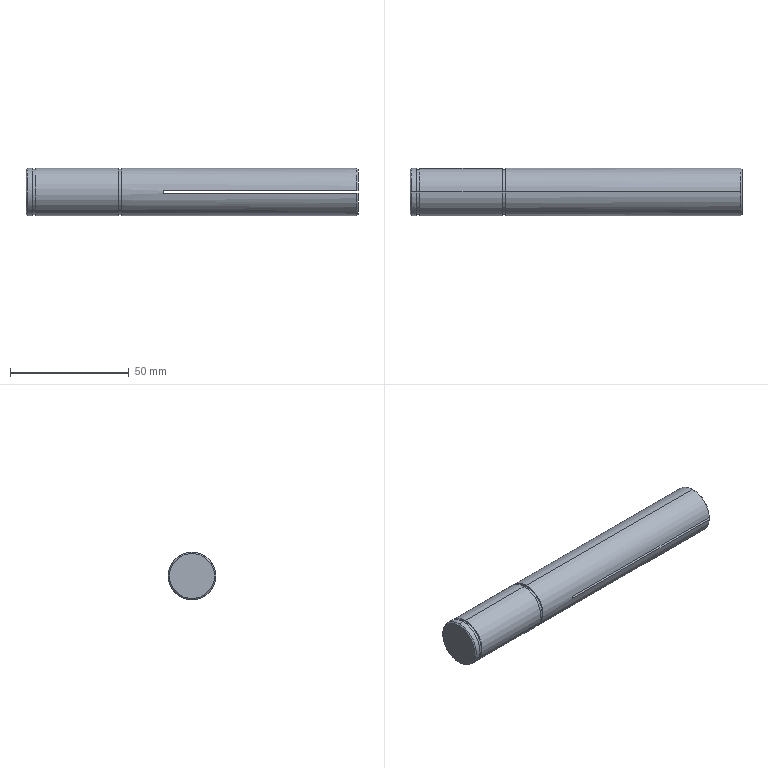Part | NX | 1 solid | 24 faces | box 140 x 20 x 20 mm | volume 42079 mm3 | plane 10 | cylinder 10 | cone 4 | commonest cylinder face diameters 20 x6 19 x4
STEP:
#1=CARTESIAN_POINT('',(0.,-9.5,0.));
#2=VERTEX_POINT('',#1);
#3=CARTESIAN_POINT('',(0.,9.5,0.));
#4=VERTEX_POINT('',#3);
#5=CARTESIAN_POINT('',(0.,0.,0.));
#6=DIRECTION('',(-1.,0.,0.));
#7=DIRECTION('',(0.,0.,-1.));
#8=AXIS2_PLACEMENT_3D('',#5,#6,#7);
#9=CIRCLE('',#8,9.5);
#10=EDGE_CURVE('',#2,#4,#9,.T.);
#11=ORIENTED_EDGE('',*,*,#10,.T.);
#12=CARTESIAN_POINT('',(0.,0.,0.));
#13=DIRECTION('',(-1.,0.,0.));
#14=DIRECTION('',(0.,0.,-1.));
#15=AXIS2_PLACEMENT_3D('',#12,#13,#14);
#16=CIRCLE('',#15,9.5);
#17=EDGE_CURVE('',#4,#2,#16,.T.);
#18=ORIENTED_EDGE('',*,*,#17,.T.);
#19=EDGE_LOOP('',(#11,#18));
#20=FACE_BOUND('',#19,.T.);
#21=CARTESIAN_POINT('',(0.,0.,0.));
#22=DIRECTION('',(1.,0.,0.));
#23=DIRECTION('',(0.,1.,0.));
#24=AXIS2_PLACEMENT_3D('',#21,#22,#23);
#25=PLANE('',#24);
#26=ADVANCED_FACE('',(#20),#25,.F.);
#27=ORIENTED_EDGE('',*,*,#10,.F.);
#28=CARTESIAN_POINT('',(0.5,-10.,0.));
#29=VERTEX_POINT('',#28);
#30=CARTESIAN_POINT('',(0.25,-9.75,0.));
#31=DIRECTION('',(0.7071,-0.7071,0.));
#32=VECTOR('',#31,1000.);
#33=LINE('',#30,#32);
#34=EDGE_CURVE('',#29,#2,#33,.F.);
#35=ORIENTED_EDGE('',*,*,#34,.F.);
#36=CARTESIAN_POINT('',(0.5,0.,10.));
#37=VERTEX_POINT('',#36);
#38=CARTESIAN_POINT('',(0.5,0.,0.));
#39=DIRECTION('',(-1.,0.,0.));
#40=DIRECTION('',(0.,0.,-1.));
#41=AXIS2_PLACEMENT_3D('',#38,#39,#40);
#42=CIRCLE('',#41,10.);
#43=EDGE_CURVE('',#29,#37,#42,.T.);
#44=ORIENTED_EDGE('',*,*,#43,.T.);
#45=CARTESIAN_POINT('',(0.5,10.,0.));
#46=VERTEX_POINT('',#45);
#47=CARTESIAN_POINT('',(0.5,0.,0.));
#48=DIRECTION('',(-1.,0.,0.));
#49=DIRECTION('',(0.,0.,-1.));
#50=AXIS2_PLACEMENT_3D('',#47,#48,#49);
#51=CIRCLE('',#50,10.);
#52=EDGE_CURVE('',#37,#46,#51,.T.);
#53=ORIENTED_EDGE('',*,*,#52,.T.);
#54=CARTESIAN_POINT('',(0.25,9.75,0.));
#55=DIRECTION('',(0.7071,0.7071,0.));
#56=VECTOR('',#55,1000.);
#57=LINE('',#54,#56);
#58=EDGE_CURVE('',#46,#4,#57,.F.);
#59=ORIENTED_EDGE('',*,*,#58,.T.);
#60=EDGE_LOOP('',(#27,#35,#44,#53,#59));
#61=FACE_BOUND('',#60,.T.);
#62=CARTESIAN_POINT('',(0.25,0.,0.));
#63=DIRECTION('',(1.,0.,0.));
#64=DIRECTION('',(0.,-1.,0.));
#65=AXIS2_PLACEMENT_3D('',#62,#63,#64);
#66=CONICAL_SURFACE('',#65,9.75,0.7854);
#67=ADVANCED_FACE('',(#61),#66,.T.);
#68=CARTESIAN_POINT('',(2.65,0.,-10.));
#69=VERTEX_POINT('',#68);
#70=CARTESIAN_POINT('',(2.65,0.,10.));
#71=VERTEX_POINT('',#70);
#72=CARTESIAN_POINT('',(2.65,0.,0.));
#73=DIRECTION('',(1.,0.,0.));
#74=DIRECTION('',(0.,0.,1.));
#75=AXIS2_PLACEMENT_3D('',#72,#73,#74);
#76=CIRCLE('',#75,10.);
#77=EDGE_CURVE('',#69,#71,#76,.T.);
#78=ORIENTED_EDGE('',*,*,#77,.F.);
#79=CARTESIAN_POINT('',(0.5,0.,-10.));
#80=VERTEX_POINT('',#79);
#81=CARTESIAN_POINT('',(147.,0.,-10.));
#82=DIRECTION('',(-1.,0.,0.));
#83=VECTOR('',#82,1000.);
#84=LINE('',#81,#83);
#85=EDGE_CURVE('',#80,#69,#84,.F.);
#86=ORIENTED_EDGE('',*,*,#85,.F.);
#87=CARTESIAN_POINT('',(0.5,0.,0.));
#88=DIRECTION('',(-1.,0.,0.));
#89=DIRECTION('',(0.,0.,-1.));
#90=AXIS2_PLACEMENT_3D('',#87,#88,#89);
#91=CIRCLE('',#90,10.);
#92=EDGE_CURVE('',#46,#80,#91,.T.);
#93=ORIENTED_EDGE('',*,*,#92,.F.);
#94=ORIENTED_EDGE('',*,*,#52,.F.);
#95=CARTESIAN_POINT('',(147.,0.,10.));
#96=DIRECTION('',(-1.,0.,0.));
#97=VECTOR('',#96,1000.);
#98=LINE('',#95,#97);
#99=EDGE_CURVE('',#37,#71,#98,.F.);
#100=ORIENTED_EDGE('',*,*,#99,.T.);
#101=EDGE_LOOP('',(#78,#86,#93,#94,#100));
#102=FACE_BOUND('',#101,.T.);
#103=CARTESIAN_POINT('',(147.,0.,0.));
#104=DIRECTION('',(-1.,0.,0.));
#105=DIRECTION('',(0.,0.,-1.));
#106=AXIS2_PLACEMENT_3D('',#103,#104,#105);
#107=CYLINDRICAL_SURFACE('',#106,10.);
#108=ADVANCED_FACE('',(#102),#107,.T.);
#109=CARTESIAN_POINT('',(140.,-9.484,-0.55));
#110=VERTEX_POINT('',#109);
#111=CARTESIAN_POINT('',(140.,9.484,-0.55));
#112=VERTEX_POINT('',#111);
#113=CARTESIAN_POINT('',(140.,0.,-0.55));
#114=DIRECTION('',(0.,1.,0.));
#115=VECTOR('',#114,1000.);
#116=LINE('',#113,#115);
#117=EDGE_CURVE('',#110,#112,#116,.T.);
#118=ORIENTED_EDGE('',*,*,#117,.F.);
#119=CARTESIAN_POINT('',(140.,0.,0.));
#120=DIRECTION('',(1.,0.,0.));
#121=DIRECTION('',(0.,1.,0.));
#122=AXIS2_PLACEMENT_3D('',#119,#120,#121);
#123=CIRCLE('',#122,9.5);
#124=EDGE_CURVE('',#110,#112,#123,.T.);
#125=ORIENTED_EDGE('',*,*,#124,.T.);
#126=EDGE_LOOP('',(#118,#125));
#127=FACE_BOUND('',#126,.T.);
#128=CARTESIAN_POINT('',(140.,0.,0.));
#129=DIRECTION('',(1.,0.,0.));
#130=DIRECTION('',(0.,1.,0.));
#131=AXIS2_PLACEMENT_3D('',#128,#129,#130);
#132=PLANE('',#131);
#133=ADVANCED_FACE('',(#127),#132,.T.);
#134=CARTESIAN_POINT('',(140.,9.484,0.55));
#135=VERTEX_POINT('',#134);
#136=CARTESIAN_POINT('',(140.,-9.484,0.55));
#137=VERTEX_POINT('',#136);
#138=CARTESIAN_POINT('',(140.,0.,0.55));
#139=DIRECTION('',(0.,-1.,0.));
#140=VECTOR('',#139,1000.);
#141=LINE('',#138,#140);
#142=EDGE_CURVE('',#135,#137,#141,.T.);
#143=ORIENTED_EDGE('',*,*,#142,.F.);
#144=CARTESIAN_POINT('',(140.,0.,0.));
#145=DIRECTION('',(1.,0.,0.));
#146=DIRECTION('',(0.,1.,0.));
#147=AXIS2_PLACEMENT_3D('',#144,#145,#146);
#148=CIRCLE('',#147,9.5);
#149=EDGE_CURVE('',#135,#137,#148,.T.);
#150=ORIENTED_EDGE('',*,*,#149,.T.);
#151=EDGE_LOOP('',(#143,#150));
#152=FACE_BOUND('',#151,.T.);
#153=CARTESIAN_POINT('',(140.,0.,0.));
#154=DIRECTION('',(1.,0.,0.));
#155=DIRECTION('',(0.,1.,0.));
#156=AXIS2_PLACEMENT_3D('',#153,#154,#155);
#157=PLANE('',#156);
#158=ADVANCED_FACE('',(#152),#157,.T.);
#159=ORIENTED_EDGE('',*,*,#77,.T.);
#160=CARTESIAN_POINT('',(2.65,0.,0.));
#161=DIRECTION('',(1.,0.,0.));
#162=DIRECTION('',(0.,0.,1.));
#163=AXIS2_PLACEMENT_3D('',#160,#161,#162);
#164=CIRCLE('',#163,10.);
#165=EDGE_CURVE('',#71,#69,#164,.T.);
#166=ORIENTED_EDGE('',*,*,#165,.T.);
#167=EDGE_LOOP('',(#159,#166));
#168=FACE_BOUND('',#167,.T.);
#169=CARTESIAN_POINT('',(2.65,0.,-9.5));
#170=VERTEX_POINT('',#169);
#171=CARTESIAN_POINT('',(2.65,0.,9.5));
#172=VERTEX_POINT('',#171);
#173=CARTESIAN_POINT('',(2.65,0.,0.));
#174=DIRECTION('',(-1.,0.,0.));
#175=DIRECTION('',(0.,0.,-1.));
#176=AXIS2_PLACEMENT_3D('',#173,#174,#175);
#177=CIRCLE('',#176,9.5);
#178=EDGE_CURVE('',#170,#172,#177,.T.);
#179=ORIENTED_EDGE('',*,*,#178,.T.);
#180=CARTESIAN_POINT('',(2.65,0.,0.));
#181=DIRECTION('',(-1.,0.,0.));
#182=DIRECTION('',(0.,0.,-1.));
#183=AXIS2_PLACEMENT_3D('',#180,#181,#182);
#184=CIRCLE('',#183,9.5);
#185=EDGE_CURVE('',#172,#170,#184,.T.);
#186=ORIENTED_EDGE('',*,*,#185,.T.);
#187=EDGE_LOOP('',(#179,#186));
#188=FACE_BOUND('',#187,.T.);
#189=CARTESIAN_POINT('',(2.65,0.,0.));
#190=DIRECTION('',(1.,0.,0.));
#191=DIRECTION('',(0.,1.,0.));
#192=AXIS2_PLACEMENT_3D('',#189,#190,#191);
#193=PLANE('',#192);
#194=ADVANCED_FACE('',(#168,#188),#193,.T.);
#195=ORIENTED_EDGE('',*,*,#178,.F.);
#196=CARTESIAN_POINT('',(4.,0.,-9.5));
#197=VERTEX_POINT('',#196);
#198=CARTESIAN_POINT('',(147.,0.,-9.5));
#199=DIRECTION('',(-1.,0.,0.));
#200=VECTOR('',#199,1000.);
#201=LINE('',#198,#200);
#202=EDGE_CURVE('',#170,#197,#201,.F.);
#203=ORIENTED_EDGE('',*,*,#202,.T.);
#204=CARTESIAN_POINT('',(4.,0.,9.5));
#205=VERTEX_POINT('',#204);
#206=CARTESIAN_POINT('',(4.,0.,0.));
#207=DIRECTION('',(1.,0.,0.));
#208=DIRECTION('',(0.,0.,1.));
#209=AXIS2_PLACEMENT_3D('',#206,#207,#208);
#210=CIRCLE('',#209,9.5);
#211=EDGE_CURVE('',#205,#197,#210,.T.);
#212=ORIENTED_EDGE('',*,*,#211,.F.);
#213=CARTESIAN_POINT('',(147.,0.,9.5));
#214=DIRECTION('',(-1.,0.,0.));
#215=VECTOR('',#214,1000.);
#216=LINE('',#213,#215);
#217=EDGE_CURVE('',#172,#205,#216,.F.);
#218=ORIENTED_EDGE('',*,*,#217,.F.);
#219=EDGE_LOOP('',(#195,#203,#212,#218));
#220=FACE_BOUND('',#219,.T.);
#221=CARTESIAN_POINT('',(147.,0.,0.));
#222=DIRECTION('',(-1.,0.,0.));
#223=DIRECTION('',(0.,0.,-1.));
#224=AXIS2_PLACEMENT_3D('',#221,#222,#223);
#225=CYLINDRICAL_SURFACE('',#224,9.5);
#226=ADVANCED_FACE('',(#220),#225,.T.);
#227=CARTESIAN_POINT('',(139.5,-9.985,0.55));
#228=VERTEX_POINT('',#227);
#229=CARTESIAN_POINT('',(139.5,-9.985,0.55));
#230=CARTESIAN_POINT('',(139.542,-9.943,0.55));
#231=CARTESIAN_POINT('',(139.583,-9.901,0.55));
#232=CARTESIAN_POINT('',(139.625,-9.86,0.55));
#233=CARTESIAN_POINT('',(139.667,-9.818,0.55));
#234=CARTESIAN_POINT('',(139.708,-9.776,0.55));
#235=CARTESIAN_POINT('',(139.75,-9.734,0.55));
#236=CARTESIAN_POINT('',(139.792,-9.693,0.55));
#237=CARTESIAN_POINT('',(139.833,-9.651,0.55));
#238=CARTESIAN_POINT('',(139.875,-9.609,0.55));
#239=CARTESIAN_POINT('',(139.917,-9.568,0.55));
#240=CARTESIAN_POINT('',(139.958,-9.526,0.55));
#241=CARTESIAN_POINT('',(140.,-9.484,0.55));
#242=B_SPLINE_CURVE_WITH_KNOTS('',3,(#229,#230,#231,#232,#233,#234,#235,#236,#237,#238,#239,#240,#241),.UNSPECIFIED.,.F.,.F.,(4,3,3,3,4),(0.,0.1769,0.3538,0.5308,0.7077),.UNSPECIFIED.);
#243=EDGE_CURVE('',#228,#137,#242,.T.);
#244=ORIENTED_EDGE('',*,*,#243,.F.);
#245=CARTESIAN_POINT('',(57.9,-9.985,0.55));
#246=VERTEX_POINT('',#245);
#247=CARTESIAN_POINT('',(147.,-9.985,0.55));
#248=DIRECTION('',(-1.,0.,0.));
#249=VECTOR('',#248,1000.);
#250=LINE('',#247,#249);
#251=EDGE_CURVE('',#228,#246,#250,.T.);
#252=ORIENTED_EDGE('',*,*,#251,.T.);
#253=CARTESIAN_POINT('',(57.9,9.985,0.55));
#254=VERTEX_POINT('',#253);
#255=CARTESIAN_POINT('',(57.9,0.,0.55));
#256=DIRECTION('',(0.,-1.,0.));
#257=VECTOR('',#256,1000.);
#258=LINE('',#255,#257);
#259=EDGE_CURVE('',#254,#246,#258,.T.);
#260=ORIENTED_EDGE('',*,*,#259,.F.);
#261=CARTESIAN_POINT('',(139.5,9.985,0.55));
#262=VERTEX_POINT('',#261);
#263=CARTESIAN_POINT('',(147.,9.985,0.55));
#264=DIRECTION('',(-1.,0.,0.));
#265=VECTOR('',#264,1000.);
#266=LINE('',#263,#265);
#267=EDGE_CURVE('',#262,#254,#266,.T.);
#268=ORIENTED_EDGE('',*,*,#267,.F.);
#269=CARTESIAN_POINT('',(140.,9.484,0.55));
#270=CARTESIAN_POINT('',(139.958,9.526,0.55));
#271=CARTESIAN_POINT('',(139.917,9.568,0.55));
#272=CARTESIAN_POINT('',(139.875,9.609,0.55));
#273=CARTESIAN_POINT('',(139.833,9.651,0.55));
#274=CARTESIAN_POINT('',(139.792,9.693,0.55));
#275=CARTESIAN_POINT('',(139.75,9.734,0.55));
#276=CARTESIAN_POINT('',(139.708,9.776,0.55));
#277=CARTESIAN_POINT('',(139.667,9.818,0.55));
#278=CARTESIAN_POINT('',(139.625,9.86,0.55));
#279=CARTESIAN_POINT('',(139.583,9.901,0.55));
#280=CARTESIAN_POINT('',(139.542,9.943,0.55));
#281=CARTESIAN_POINT('',(139.5,9.985,0.55));
#282=B_SPLINE_CURVE_WITH_KNOTS('',3,(#269,#270,#271,#272,#273,#274,#275,#276,#277,#278,#279,#280,#281),.UNSPECIFIED.,.F.,.F.,(4,3,3,3,4),(0.,0.1769,0.3538,0.5308,0.7077),.UNSPECIFIED.);
#283=EDGE_CURVE('',#135,#262,#282,.T.);
#284=ORIENTED_EDGE('',*,*,#283,.F.);
#285=ORIENTED_EDGE('',*,*,#142,.T.);
#286=EDGE_LOOP('',(#244,#252,#260,#268,#284,#285));
#287=FACE_BOUND('',#286,.T.);
#288=CARTESIAN_POINT('',(140.,-10.978,0.55));
#289=DIRECTION('',(0.,0.,-1.));
#290=DIRECTION('',(0.,-1.,0.));
#291=AXIS2_PLACEMENT_3D('',#288,#289,#290);
#292=PLANE('',#291);
#293=ADVANCED_FACE('',(#287),#292,.T.);
#294=CARTESIAN_POINT('',(4.,0.,10.));
#295=VERTEX_POINT('',#294);
#296=CARTESIAN_POINT('',(4.,0.,-10.));
#297=VERTEX_POINT('',#296);
#298=CARTESIAN_POINT('',(4.,0.,0.));
#299=DIRECTION('',(-1.,0.,0.));
#300=DIRECTION('',(0.,0.,-1.));
#301=AXIS2_PLACEMENT_3D('',#298,#299,#300);
#302=CIRCLE('',#301,10.);
#303=EDGE_CURVE('',#295,#297,#302,.T.);
#304=ORIENTED_EDGE('',*,*,#303,.T.);
#305=CARTESIAN_POINT('',(4.,0.,0.));
#306=DIRECTION('',(-1.,0.,0.));
#307=DIRECTION('',(0.,0.,-1.));
#308=AXIS2_PLACEMENT_3D('',#305,#306,#307);
#309=CIRCLE('',#308,10.);
#310=EDGE_CURVE('',#297,#295,#309,.T.);
#311=ORIENTED_EDGE('',*,*,#310,.T.);
#312=EDGE_LOOP('',(#304,#311));
#313=FACE_BOUND('',#312,.T.);
#314=CARTESIAN_POINT('',(4.,0.,0.));
#315=DIRECTION('',(1.,0.,0.));
#316=DIRECTION('',(0.,0.,1.));
#317=AXIS2_PLACEMENT_3D('',#314,#315,#316);
#318=CIRCLE('',#317,9.5);
#319=EDGE_CURVE('',#197,#205,#318,.T.);
#320=ORIENTED_EDGE('',*,*,#319,.T.);
#321=ORIENTED_EDGE('',*,*,#211,.T.);
#322=EDGE_LOOP('',(#320,#321));
#323=FACE_BOUND('',#322,.T.);
#324=CARTESIAN_POINT('',(4.,0.,0.));
#325=DIRECTION('',(1.,0.,0.));
#326=DIRECTION('',(0.,1.,0.));
#327=AXIS2_PLACEMENT_3D('',#324,#325,#326);
#328=PLANE('',#327);
#329=ADVANCED_FACE('',(#313,#323),#328,.F.);
#330=ORIENTED_EDGE('',*,*,#303,.F.);
#331=CARTESIAN_POINT('',(39.,0.,10.));
#332=VERTEX_POINT('',#331);
#333=CARTESIAN_POINT('',(147.,0.,10.));
#334=DIRECTION('',(-1.,0.,0.));
#335=VECTOR('',#334,1000.);
#336=LINE('',#333,#335);
#337=EDGE_CURVE('',#332,#295,#336,.T.);
#338=ORIENTED_EDGE('',*,*,#337,.F.);
#339=CARTESIAN_POINT('',(39.,0.,-10.));
#340=VERTEX_POINT('',#339);
#341=CARTESIAN_POINT('',(39.,0.,0.));
#342=DIRECTION('',(1.,0.,0.));
#343=DIRECTION('',(0.,0.,1.));
#344=AXIS2_PLACEMENT_3D('',#341,#342,#343);
#345=CIRCLE('',#344,10.);
#346=EDGE_CURVE('',#340,#332,#345,.T.);
#347=ORIENTED_EDGE('',*,*,#346,.F.);
#348=CARTESIAN_POINT('',(147.,0.,-10.));
#349=DIRECTION('',(-1.,0.,0.));
#350=VECTOR('',#349,1000.);
#351=LINE('',#348,#350);
#352=EDGE_CURVE('',#340,#297,#351,.T.);
#353=ORIENTED_EDGE('',*,*,#352,.T.);
#354=EDGE_LOOP('',(#330,#338,#347,#353));
#355=FACE_BOUND('',#354,.T.);
#356=CARTESIAN_POINT('',(147.,0.,0.));
#357=DIRECTION('',(-1.,0.,0.));
#358=DIRECTION('',(0.,0.,-1.));
#359=AXIS2_PLACEMENT_3D('',#356,#357,#358);
#360=CYLINDRICAL_SURFACE('',#359,10.);
#361=ADVANCED_FACE('',(#355),#360,.T.);
#362=CARTESIAN_POINT('',(139.5,9.985,-0.55));
#363=VERTEX_POINT('',#362);
#364=CARTESIAN_POINT('',(139.5,9.985,-0.55));
#365=CARTESIAN_POINT('',(139.542,9.943,-0.55));
#366=CARTESIAN_POINT('',(139.583,9.901,-0.55));
#367=CARTESIAN_POINT('',(139.625,9.86,-0.55));
#368=CARTESIAN_POINT('',(139.667,9.818,-0.55));
#369=CARTESIAN_POINT('',(139.708,9.776,-0.55));
#370=CARTESIAN_POINT('',(139.75,9.734,-0.55));
#371=CARTESIAN_POINT('',(139.792,9.693,-0.55));
#372=CARTESIAN_POINT('',(139.833,9.651,-0.55));
#373=CARTESIAN_POINT('',(139.875,9.609,-0.55));
#374=CARTESIAN_POINT('',(139.917,9.568,-0.55));
#375=CARTESIAN_POINT('',(139.958,9.526,-0.55));
#376=CARTESIAN_POINT('',(140.,9.484,-0.55));
#377=B_SPLINE_CURVE_WITH_KNOTS('',3,(#364,#365,#366,#367,#368,#369,#370,#371,#372,#373,#374,#375,#376),.UNSPECIFIED.,.F.,.F.,(4,3,3,3,4),(0.,0.1769,0.3538,0.5308,0.7077),.UNSPECIFIED.);
#378=EDGE_CURVE('',#363,#112,#377,.T.);
#379=ORIENTED_EDGE('',*,*,#378,.F.);
#380=CARTESIAN_POINT('',(57.9,9.985,-0.55));
#381=VERTEX_POINT('',#380);
#382=CARTESIAN_POINT('',(147.,9.985,-0.55));
#383=DIRECTION('',(-1.,0.,0.));
#384=VECTOR('',#383,1000.);
#385=LINE('',#382,#384);
#386=EDGE_CURVE('',#363,#381,#385,.T.);
#387=ORIENTED_EDGE('',*,*,#386,.T.);
#388=CARTESIAN_POINT('',(57.9,-9.985,-0.55));
#389=VERTEX_POINT('',#388);
#390=CARTESIAN_POINT('',(57.9,0.,-0.55));
#391=DIRECTION('',(0.,1.,0.));
#392=VECTOR('',#391,1000.);
#393=LINE('',#390,#392);
#394=EDGE_CURVE('',#389,#381,#393,.T.);
#395=ORIENTED_EDGE('',*,*,#394,.F.);
#396=CARTESIAN_POINT('',(139.5,-9.985,-0.55));
#397=VERTEX_POINT('',#396);
#398=CARTESIAN_POINT('',(147.,-9.985,-0.55));
#399=DIRECTION('',(-1.,0.,0.));
#400=VECTOR('',#399,1000.);
#401=LINE('',#398,#400);
#402=EDGE_CURVE('',#397,#389,#401,.T.);
#403=ORIENTED_EDGE('',*,*,#402,.F.);
#404=CARTESIAN_POINT('',(140.,-9.484,-0.55));
#405=CARTESIAN_POINT('',(139.958,-9.526,-0.55));
#406=CARTESIAN_POINT('',(139.917,-9.568,-0.55));
#407=CARTESIAN_POINT('',(139.875,-9.609,-0.55));
#408=CARTESIAN_POINT('',(139.833,-9.651,-0.55));
#409=CARTESIAN_POINT('',(139.792,-9.693,-0.55));
#410=CARTESIAN_POINT('',(139.75,-9.734,-0.55));
#411=CARTESIAN_POINT('',(139.708,-9.776,-0.55));
#412=CARTESIAN_POINT('',(139.667,-9.818,-0.55));
#413=CARTESIAN_POINT('',(139.625,-9.86,-0.55));
#414=CARTESIAN_POINT('',(139.583,-9.901,-0.55));
#415=CARTESIAN_POINT('',(139.542,-9.943,-0.55));
#416=CARTESIAN_POINT('',(139.5,-9.985,-0.55));
#417=B_SPLINE_CURVE_WITH_KNOTS('',3,(#404,#405,#406,#407,#408,#409,#410,#411,#412,#413,#414,#415,#416),.UNSPECIFIED.,.F.,.F.,(4,3,3,3,4),(0.,0.1769,0.3538,0.5308,0.7077),.UNSPECIFIED.);
#418=EDGE_CURVE('',#110,#397,#417,.T.);
#419=ORIENTED_EDGE('',*,*,#418,.F.);
#420=ORIENTED_EDGE('',*,*,#117,.T.);
#421=EDGE_LOOP('',(#379,#387,#395,#403,#419,#420));
#422=FACE_BOUND('',#421,.T.);
#423=CARTESIAN_POINT('',(140.,11.845,-0.55));
#424=DIRECTION('',(0.,0.,1.));
#425=DIRECTION('',(1.,0.,0.));
#426=AXIS2_PLACEMENT_3D('',#423,#424,#425);
#427=PLANE('',#426);
#428=ADVANCED_FACE('',(#422),#427,.T.);
#429=CARTESIAN_POINT('',(39.,0.,0.));
#430=DIRECTION('',(1.,0.,0.));
#431=DIRECTION('',(0.,0.,1.));
#432=AXIS2_PLACEMENT_3D('',#429,#430,#431);
#433=CIRCLE('',#432,10.);
#434=EDGE_CURVE('',#332,#340,#433,.T.);
#435=ORIENTED_EDGE('',*,*,#434,.T.);
#436=ORIENTED_EDGE('',*,*,#346,.T.);
#437=EDGE_LOOP('',(#435,#436));
#438=FACE_BOUND('',#437,.T.);
#439=CARTESIAN_POINT('',(39.,0.,-9.5));
#440=VERTEX_POINT('',#439);
#441=CARTESIAN_POINT('',(39.,0.,9.5));
#442=VERTEX_POINT('',#441);
#443=CARTESIAN_POINT('',(39.,0.,0.));
#444=DIRECTION('',(-1.,0.,0.));
#445=DIRECTION('',(0.,0.,-1.));
#446=AXIS2_PLACEMENT_3D('',#443,#444,#445);
#447=CIRCLE('',#446,9.5);
#448=EDGE_CURVE('',#440,#442,#447,.T.);
#449=ORIENTED_EDGE('',*,*,#448,.T.);
#450=CARTESIAN_POINT('',(39.,0.,0.));
#451=DIRECTION('',(-1.,0.,0.));
#452=DIRECTION('',(0.,0.,-1.));
#453=AXIS2_PLACEMENT_3D('',#450,#451,#452);
#454=CIRCLE('',#453,9.5);
#455=EDGE_CURVE('',#442,#440,#454,.T.);
#456=ORIENTED_EDGE('',*,*,#455,.T.);
#457=EDGE_LOOP('',(#449,#456));
#458=FACE_BOUND('',#457,.T.);
#459=CARTESIAN_POINT('',(39.,0.,0.));
#460=DIRECTION('',(1.,0.,0.));
#461=DIRECTION('',(0.,1.,0.));
#462=AXIS2_PLACEMENT_3D('',#459,#460,#461);
#463=PLANE('',#462);
#464=ADVANCED_FACE('',(#438,#458),#463,.T.);
#465=ORIENTED_EDGE('',*,*,#448,.F.);
#466=CARTESIAN_POINT('',(40.35,0.,-9.5));
#467=VERTEX_POINT('',#466);
#468=CARTESIAN_POINT('',(147.,0.,-9.5));
#469=DIRECTION('',(-1.,0.,0.));
#470=VECTOR('',#469,1000.);
#471=LINE('',#468,#470);
#472=EDGE_CURVE('',#440,#467,#471,.F.);
#473=ORIENTED_EDGE('',*,*,#472,.T.);
#474=CARTESIAN_POINT('',(40.35,0.,9.5));
#475=VERTEX_POINT('',#474);
#476=CARTESIAN_POINT('',(40.35,0.,0.));
#477=DIRECTION('',(1.,0.,0.));
#478=DIRECTION('',(0.,0.,-1.));
#479=AXIS2_PLACEMENT_3D('',#476,#477,#478);
#480=CIRCLE('',#479,9.5);
#481=EDGE_CURVE('',#475,#467,#480,.T.);
#482=ORIENTED_EDGE('',*,*,#481,.F.);
#483=CARTESIAN_POINT('',(147.,0.,9.5));
#484=DIRECTION('',(-1.,0.,0.));
#485=VECTOR('',#484,1000.);
#486=LINE('',#483,#485);
#487=EDGE_CURVE('',#442,#475,#486,.F.);
#488=ORIENTED_EDGE('',*,*,#487,.F.);
#489=EDGE_LOOP('',(#465,#473,#482,#488));
#490=FACE_BOUND('',#489,.T.);
#491=CARTESIAN_POINT('',(147.,0.,0.));
#492=DIRECTION('',(-1.,0.,0.));
#493=DIRECTION('',(0.,0.,-1.));
#494=AXIS2_PLACEMENT_3D('',#491,#492,#493);
#495=CYLINDRICAL_SURFACE('',#494,9.5);
#496=ADVANCED_FACE('',(#490),#495,.T.);
#497=ORIENTED_EDGE('',*,*,#259,.T.);
#498=CARTESIAN_POINT('',(57.9,0.,0.));
#499=DIRECTION('',(1.,0.,0.));
#500=DIRECTION('',(0.,0.,-1.));
#501=AXIS2_PLACEMENT_3D('',#498,#499,#500);
#502=CIRCLE('',#501,10.);
#503=EDGE_CURVE('',#246,#389,#502,.T.);
#504=ORIENTED_EDGE('',*,*,#503,.T.);
#505=ORIENTED_EDGE('',*,*,#394,.T.);
#506=CARTESIAN_POINT('',(57.9,0.,0.));
#507=DIRECTION('',(1.,0.,0.));
#508=DIRECTION('',(0.,0.,-1.));
#509=AXIS2_PLACEMENT_3D('',#506,#507,#508);
#510=CIRCLE('',#509,10.);
#511=EDGE_CURVE('',#381,#254,#510,.T.);
#512=ORIENTED_EDGE('',*,*,#511,.T.);
#513=EDGE_LOOP('',(#497,#504,#505,#512));
#514=FACE_BOUND('',#513,.T.);
#515=CARTESIAN_POINT('',(57.9,0.,0.));
#516=DIRECTION('',(1.,0.,0.));
#517=DIRECTION('',(0.,1.,0.));
#518=AXIS2_PLACEMENT_3D('',#515,#516,#517);
#519=PLANE('',#518);
#520=ADVANCED_FACE('',(#514),#519,.T.);
#521=CARTESIAN_POINT('',(40.35,0.,-10.));
#522=VERTEX_POINT('',#521);
#523=CARTESIAN_POINT('',(40.35,0.,10.));
#524=VERTEX_POINT('',#523);
#525=CARTESIAN_POINT('',(40.35,0.,0.));
#526=DIRECTION('',(1.,0.,0.));
#527=DIRECTION('',(0.,0.,-1.));
#528=AXIS2_PLACEMENT_3D('',#525,#526,#527);
#529=CIRCLE('',#528,10.);
#530=EDGE_CURVE('',#522,#524,#529,.T.);
#531=ORIENTED_EDGE('',*,*,#530,.F.);
#532=CARTESIAN_POINT('',(40.35,0.,0.));
#533=DIRECTION('',(1.,0.,0.));
#534=DIRECTION('',(0.,0.,-1.));
#535=AXIS2_PLACEMENT_3D('',#532,#533,#534);
#536=CIRCLE('',#535,10.);
#537=EDGE_CURVE('',#524,#522,#536,.T.);
#538=ORIENTED_EDGE('',*,*,#537,.F.);
#539=EDGE_LOOP('',(#531,#538));
#540=FACE_BOUND('',#539,.T.);
#541=ORIENTED_EDGE('',*,*,#481,.T.);
#542=CARTESIAN_POINT('',(40.35,0.,0.));
#543=DIRECTION('',(1.,0.,0.));
#544=DIRECTION('',(0.,0.,-1.));
#545=AXIS2_PLACEMENT_3D('',#542,#543,#544);
#546=CIRCLE('',#545,9.5);
#547=EDGE_CURVE('',#467,#475,#546,.T.);
#548=ORIENTED_EDGE('',*,*,#547,.T.);
#549=EDGE_LOOP('',(#541,#548));
#550=FACE_BOUND('',#549,.T.);
#551=CARTESIAN_POINT('',(40.35,0.,0.));
#552=DIRECTION('',(1.,0.,0.));
#553=DIRECTION('',(0.,1.,0.));
#554=AXIS2_PLACEMENT_3D('',#551,#552,#553);
#555=PLANE('',#554);
#556=ADVANCED_FACE('',(#540,#550),#555,.F.);
#557=ORIENTED_EDGE('',*,*,#267,.T.);
#558=ORIENTED_EDGE('',*,*,#511,.F.);
#559=ORIENTED_EDGE('',*,*,#386,.F.);
#560=CARTESIAN_POINT('',(139.5,0.,-10.));
#561=VERTEX_POINT('',#560);
#562=CARTESIAN_POINT('',(139.5,0.,0.));
#563=DIRECTION('',(1.,0.,0.));
#564=DIRECTION('',(0.,1.,0.));
#565=AXIS2_PLACEMENT_3D('',#562,#563,#564);
#566=CIRCLE('',#565,10.);
#567=EDGE_CURVE('',#561,#363,#566,.T.);
#568=ORIENTED_EDGE('',*,*,#567,.F.);
#569=CARTESIAN_POINT('',(147.,0.,-10.));
#570=DIRECTION('',(-1.,0.,0.));
#571=VECTOR('',#570,1000.);
#572=LINE('',#569,#571);
#573=EDGE_CURVE('',#522,#561,#572,.F.);
#574=ORIENTED_EDGE('',*,*,#573,.F.);
#575=ORIENTED_EDGE('',*,*,#530,.T.);
#576=CARTESIAN_POINT('',(139.5,0.,10.));
#577=VERTEX_POINT('',#576);
#578=CARTESIAN_POINT('',(147.,0.,10.));
#579=DIRECTION('',(-1.,0.,0.));
#580=VECTOR('',#579,1000.);
#581=LINE('',#578,#580);
#582=EDGE_CURVE('',#524,#577,#581,.F.);
#583=ORIENTED_EDGE('',*,*,#582,.T.);
#584=CARTESIAN_POINT('',(139.5,0.,0.));
#585=DIRECTION('',(1.,0.,0.));
#586=DIRECTION('',(0.,1.,0.));
#587=AXIS2_PLACEMENT_3D('',#584,#585,#586);
#588=CIRCLE('',#587,10.);
#589=EDGE_CURVE('',#262,#577,#588,.T.);
#590=ORIENTED_EDGE('',*,*,#589,.F.);
#591=EDGE_LOOP('',(#557,#558,#559,#568,#574,#575,#583,#590));
#592=FACE_BOUND('',#591,.T.);
#593=CARTESIAN_POINT('',(147.,0.,0.));
#594=DIRECTION('',(-1.,0.,0.));
#595=DIRECTION('',(0.,0.,-1.));
#596=AXIS2_PLACEMENT_3D('',#593,#594,#595);
#597=CYLINDRICAL_SURFACE('',#596,10.);
#598=ADVANCED_FACE('',(#592),#597,.T.);
#599=ORIENTED_EDGE('',*,*,#243,.T.);
#600=ORIENTED_EDGE('',*,*,#149,.F.);
#601=ORIENTED_EDGE('',*,*,#283,.T.);
#602=ORIENTED_EDGE('',*,*,#589,.T.);
#603=CARTESIAN_POINT('',(139.5,0.,0.));
#604=DIRECTION('',(1.,0.,0.));
#605=DIRECTION('',(0.,1.,0.));
#606=AXIS2_PLACEMENT_3D('',#603,#604,#605);
#607=CIRCLE('',#606,10.);
#608=EDGE_CURVE('',#577,#228,#607,.T.);
#609=ORIENTED_EDGE('',*,*,#608,.T.);
#610=EDGE_LOOP('',(#599,#600,#601,#602,#609));
#611=FACE_BOUND('',#610,.T.);
#612=CARTESIAN_POINT('',(139.5,0.,0.));
#613=DIRECTION('',(-1.,0.,0.));
#614=DIRECTION('',(0.,1.,0.));
#615=AXIS2_PLACEMENT_3D('',#612,#613,#614);
#616=CONICAL_SURFACE('',#615,10.,0.7854);
#617=ADVANCED_FACE('',(#611),#616,.T.);
#618=ORIENTED_EDGE('',*,*,#378,.T.);
#619=ORIENTED_EDGE('',*,*,#124,.F.);
#620=ORIENTED_EDGE('',*,*,#418,.T.);
#621=CARTESIAN_POINT('',(139.5,0.,0.));
#622=DIRECTION('',(1.,0.,0.));
#623=DIRECTION('',(0.,1.,0.));
#624=AXIS2_PLACEMENT_3D('',#621,#622,#623);
#625=CIRCLE('',#624,10.);
#626=EDGE_CURVE('',#397,#561,#625,.T.);
#627=ORIENTED_EDGE('',*,*,#626,.T.);
#628=ORIENTED_EDGE('',*,*,#567,.T.);
#629=EDGE_LOOP('',(#618,#619,#620,#627,#628));
#630=FACE_BOUND('',#629,.T.);
#631=CARTESIAN_POINT('',(139.5,0.,0.));
#632=DIRECTION('',(-1.,0.,0.));
#633=DIRECTION('',(0.,1.,0.));
#634=AXIS2_PLACEMENT_3D('',#631,#632,#633);
#635=CONICAL_SURFACE('',#634,10.,0.7854);
#636=ADVANCED_FACE('',(#630),#635,.T.);
#637=ORIENTED_EDGE('',*,*,#573,.T.);
#638=ORIENTED_EDGE('',*,*,#626,.F.);
#639=ORIENTED_EDGE('',*,*,#402,.T.);
#640=ORIENTED_EDGE('',*,*,#503,.F.);
#641=ORIENTED_EDGE('',*,*,#251,.F.);
#642=ORIENTED_EDGE('',*,*,#608,.F.);
#643=ORIENTED_EDGE('',*,*,#582,.F.);
#644=ORIENTED_EDGE('',*,*,#537,.T.);
#645=EDGE_LOOP('',(#637,#638,#639,#640,#641,#642,#643,#644));
#646=FACE_BOUND('',#645,.T.);
#647=CARTESIAN_POINT('',(147.,0.,0.));
#648=DIRECTION('',(-1.,0.,0.));
#649=DIRECTION('',(0.,0.,-1.));
#650=AXIS2_PLACEMENT_3D('',#647,#648,#649);
#651=CYLINDRICAL_SURFACE('',#650,10.);
#652=ADVANCED_FACE('',(#646),#651,.T.);
#653=CARTESIAN_POINT('',(0.5,0.,0.));
#654=DIRECTION('',(-1.,0.,0.));
#655=DIRECTION('',(0.,0.,-1.));
#656=AXIS2_PLACEMENT_3D('',#653,#654,#655);
#657=CIRCLE('',#656,10.);
#658=EDGE_CURVE('',#80,#29,#657,.T.);
#659=ORIENTED_EDGE('',*,*,#658,.F.);
#660=ORIENTED_EDGE('',*,*,#85,.T.);
#661=ORIENTED_EDGE('',*,*,#165,.F.);
#662=ORIENTED_EDGE('',*,*,#99,.F.);
#663=ORIENTED_EDGE('',*,*,#43,.F.);
#664=EDGE_LOOP('',(#659,#660,#661,#662,#663));
#665=FACE_BOUND('',#664,.T.);
#666=CARTESIAN_POINT('',(147.,0.,0.));
#667=DIRECTION('',(-1.,0.,0.));
#668=DIRECTION('',(0.,0.,-1.));
#669=AXIS2_PLACEMENT_3D('',#666,#667,#668);
#670=CYLINDRICAL_SURFACE('',#669,10.);
#671=ADVANCED_FACE('',(#665),#670,.T.);
#672=ORIENTED_EDGE('',*,*,#472,.F.);
#673=ORIENTED_EDGE('',*,*,#455,.F.);
#674=ORIENTED_EDGE('',*,*,#487,.T.);
#675=ORIENTED_EDGE('',*,*,#547,.F.);
#676=EDGE_LOOP('',(#672,#673,#674,#675));
#677=FACE_BOUND('',#676,.T.);
#678=CARTESIAN_POINT('',(147.,0.,0.));
#679=DIRECTION('',(-1.,0.,0.));
#680=DIRECTION('',(0.,0.,-1.));
#681=AXIS2_PLACEMENT_3D('',#678,#679,#680);
#682=CYLINDRICAL_SURFACE('',#681,9.5);
#683=ADVANCED_FACE('',(#677),#682,.T.);
#684=ORIENTED_EDGE('',*,*,#658,.T.);
#685=ORIENTED_EDGE('',*,*,#34,.T.);
#686=ORIENTED_EDGE('',*,*,#17,.F.);
#687=ORIENTED_EDGE('',*,*,#58,.F.);
#688=ORIENTED_EDGE('',*,*,#92,.T.);
#689=EDGE_LOOP('',(#684,#685,#686,#687,#688));
#690=FACE_BOUND('',#689,.T.);
#691=CARTESIAN_POINT('',(0.25,0.,0.));
#692=DIRECTION('',(1.,0.,0.));
#693=DIRECTION('',(0.,-1.,0.));
#694=AXIS2_PLACEMENT_3D('',#691,#692,#693);
#695=CONICAL_SURFACE('',#694,9.75,0.7854);
#696=ADVANCED_FACE('',(#690),#695,.T.);
#697=ORIENTED_EDGE('',*,*,#434,.F.);
#698=ORIENTED_EDGE('',*,*,#337,.T.);
#699=ORIENTED_EDGE('',*,*,#310,.F.);
#700=ORIENTED_EDGE('',*,*,#352,.F.);
#701=EDGE_LOOP('',(#697,#698,#699,#700));
#702=FACE_BOUND('',#701,.T.);
#703=CARTESIAN_POINT('',(147.,0.,0.));
#704=DIRECTION('',(-1.,0.,0.));
#705=DIRECTION('',(0.,0.,-1.));
#706=AXIS2_PLACEMENT_3D('',#703,#704,#705);
#707=CYLINDRICAL_SURFACE('',#706,10.);
#708=ADVANCED_FACE('',(#702),#707,.T.);
#709=ORIENTED_EDGE('',*,*,#319,.F.);
#710=ORIENTED_EDGE('',*,*,#202,.F.);
#711=ORIENTED_EDGE('',*,*,#185,.F.);
#712=ORIENTED_EDGE('',*,*,#217,.T.);
#713=EDGE_LOOP('',(#709,#710,#711,#712));
#714=FACE_BOUND('',#713,.T.);
#715=CARTESIAN_POINT('',(147.,0.,0.));
#716=DIRECTION('',(-1.,0.,0.));
#717=DIRECTION('',(0.,0.,-1.));
#718=AXIS2_PLACEMENT_3D('',#715,#716,#717);
#719=CYLINDRICAL_SURFACE('',#718,9.5);
#720=ADVANCED_FACE('',(#714),#719,.T.);
#721=CLOSED_SHELL('',(#26,#67,#108,#133,#158,#194,#226,#293,#329,#361,#428,#464,#496,#520,#556,#598,#617,#636,#652,#671,#683,#696,#708,#720));
#722=MANIFOLD_SOLID_BREP('',#721);
#723=(LENGTH_UNIT()NAMED_UNIT(*)SI_UNIT(.MILLI.,.METRE.));
#724=UNCERTAINTY_MEASURE_WITH_UNIT(LENGTH_MEASURE(0.00001),#723,'','');
#725=(NAMED_UNIT(*)PLANE_ANGLE_UNIT()SI_UNIT($,.RADIAN.));
#726=(NAMED_UNIT(*)SI_UNIT($,.STERADIAN.)SOLID_ANGLE_UNIT());
#727=(GEOMETRIC_REPRESENTATION_CONTEXT(3)GLOBAL_UNCERTAINTY_ASSIGNED_CONTEXT((#724))GLOBAL_UNIT_ASSIGNED_CONTEXT((#723,#725,#726))REPRESENTATION_CONTEXT('',''));
#728=ADVANCED_BREP_SHAPE_REPRESENTATION('',(#722),#727);